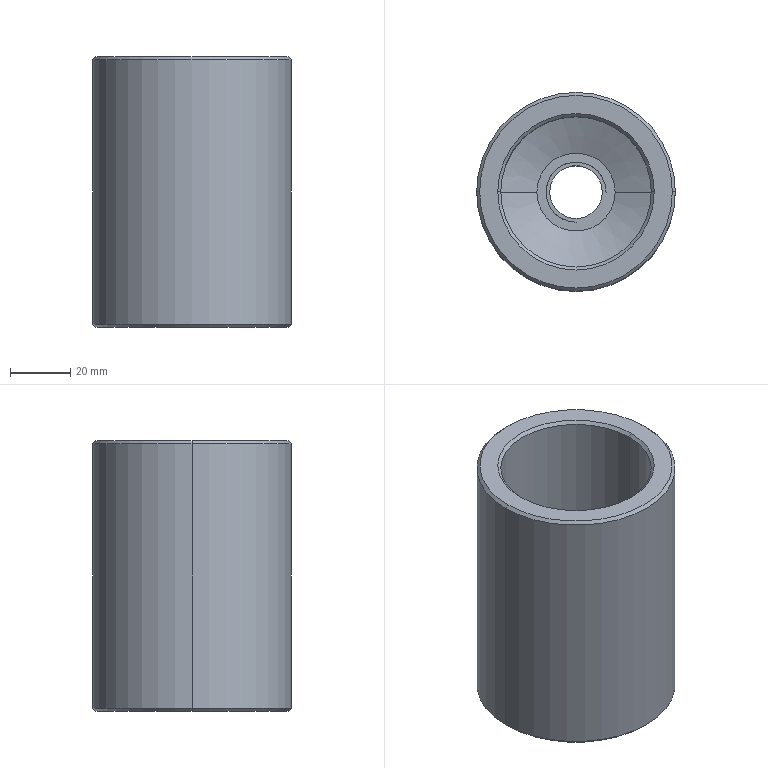Part | Creo | 1 solid | 21 faces | box 66 x 66 x 90 mm | volume 165854 mm3 | cone 8 | cylinder 8 | plane 5 | commonest cylinder face diameters 17.5 x2 50 x2 66 x2 19.94 x1 20 x1
STEP:
#1=CARTESIAN_POINT('',(-203.,-292.005,-366.));
#2=VERTEX_POINT('',#1);
#3=CARTESIAN_POINT('',(-267.,-292.005,-366.));
#4=VERTEX_POINT('',#3);
#5=CARTESIAN_POINT('',(-235.,-292.005,-366.));
#6=DIRECTION('',(0.,0.,-1.));
#7=DIRECTION('',(1.,0.,0.));
#8=AXIS2_PLACEMENT_3D('',#5,#6,#7);
#9=CIRCLE('',#8,32.);
#10=EDGE_CURVE('',#2,#4,#9,.T.);
#11=ORIENTED_EDGE('',*,*,#10,.F.);
#12=CARTESIAN_POINT('',(-235.,-292.005,-366.));
#13=DIRECTION('',(0.,0.,-1.));
#14=DIRECTION('',(-1.,0.,0.));
#15=AXIS2_PLACEMENT_3D('',#12,#13,#14);
#16=CIRCLE('',#15,32.);
#17=EDGE_CURVE('',#4,#2,#16,.T.);
#18=ORIENTED_EDGE('',*,*,#17,.F.);
#19=EDGE_LOOP('',(#11,#18));
#20=FACE_OUTER_BOUND('',#19,.F.);
#21=CARTESIAN_POINT('',(-225.03,-292.005,-366.));
#22=VERTEX_POINT('',#21);
#23=CARTESIAN_POINT('',(-225.,-292.005,-366.));
#24=VERTEX_POINT('',#23);
#25=CARTESIAN_POINT('',(-225.03,-292.005,-366.));
#26=DIRECTION('',(1.,0.,0.));
#27=VECTOR('',#26,0.03);
#28=LINE('',#25,#27);
#29=EDGE_CURVE('',#22,#24,#28,.T.);
#30=ORIENTED_EDGE('',*,*,#29,.F.);
#31=CARTESIAN_POINT('',(-244.97,-292.005,-366.));
#32=VERTEX_POINT('',#31);
#33=CARTESIAN_POINT('',(-235.,-292.005,-366.));
#34=DIRECTION('',(0.,0.,-1.));
#35=DIRECTION('',(-1.,0.,0.));
#36=AXIS2_PLACEMENT_3D('',#33,#34,#35);
#37=CIRCLE('',#36,9.97);
#38=EDGE_CURVE('',#32,#22,#37,.T.);
#39=ORIENTED_EDGE('',*,*,#38,.F.);
#40=CARTESIAN_POINT('',(-235.,-301.975,-366.));
#41=VERTEX_POINT('',#40);
#42=CARTESIAN_POINT('',(-235.,-292.005,-366.));
#43=DIRECTION('',(0.,0.,-1.));
#44=DIRECTION('',(0.,-1.,0.));
#45=AXIS2_PLACEMENT_3D('',#42,#43,#44);
#46=CIRCLE('',#45,9.97);
#47=EDGE_CURVE('',#41,#32,#46,.T.);
#48=ORIENTED_EDGE('',*,*,#47,.F.);
#49=CARTESIAN_POINT('',(-235.,-302.005,-366.));
#50=VERTEX_POINT('',#49);
#51=CARTESIAN_POINT('',(-235.,-302.005,-366.));
#52=DIRECTION('',(0.,1.,0.));
#53=VECTOR('',#52,0.03);
#54=LINE('',#51,#53);
#55=EDGE_CURVE('',#50,#41,#54,.T.);
#56=ORIENTED_EDGE('',*,*,#55,.F.);
#57=CARTESIAN_POINT('',(-245.,-292.005,-366.));
#58=VERTEX_POINT('',#57);
#59=CARTESIAN_POINT('',(-235.,-292.005,-366.));
#60=DIRECTION('',(0.,0.,1.));
#61=DIRECTION('',(-1.,0.,0.));
#62=AXIS2_PLACEMENT_3D('',#59,#60,#61);
#63=CIRCLE('',#62,10.);
#64=EDGE_CURVE('',#58,#50,#63,.T.);
#65=ORIENTED_EDGE('',*,*,#64,.F.);
#66=CARTESIAN_POINT('',(-235.,-292.005,-366.));
#67=DIRECTION('',(0.,0.,1.));
#68=DIRECTION('',(1.,0.,0.));
#69=AXIS2_PLACEMENT_3D('',#66,#67,#68);
#70=CIRCLE('',#69,10.);
#71=EDGE_CURVE('',#24,#58,#70,.T.);
#72=ORIENTED_EDGE('',*,*,#71,.F.);
#73=EDGE_LOOP('',(#30,#39,#48,#56,#65,#72));
#74=FACE_BOUND('',#73,.F.);
#75=CARTESIAN_POINT('',(-226.25,-292.005,-366.));
#76=VERTEX_POINT('',#75);
#77=CARTESIAN_POINT('',(-243.75,-292.005,-366.));
#78=VERTEX_POINT('',#77);
#79=CARTESIAN_POINT('',(-235.,-292.005,-366.));
#80=DIRECTION('',(0.,0.,1.));
#81=DIRECTION('',(1.,0.,0.));
#82=AXIS2_PLACEMENT_3D('',#79,#80,#81);
#83=CIRCLE('',#82,8.75);
#84=EDGE_CURVE('',#76,#78,#83,.T.);
#85=ORIENTED_EDGE('',*,*,#84,.F.);
#86=CARTESIAN_POINT('',(-235.,-292.005,-366.));
#87=DIRECTION('',(0.,0.,1.));
#88=DIRECTION('',(-1.,0.,0.));
#89=AXIS2_PLACEMENT_3D('',#86,#87,#88);
#90=CIRCLE('',#89,8.75);
#91=EDGE_CURVE('',#78,#76,#90,.T.);
#92=ORIENTED_EDGE('',*,*,#91,.F.);
#93=EDGE_LOOP('',(#85,#92));
#94=FACE_BOUND('',#93,.F.);
#95=CARTESIAN_POINT('',(-45.,-44.005,-366.));
#96=DIRECTION('',(0.,0.,-1.));
#97=DIRECTION('',(1.,0.,0.));
#98=AXIS2_PLACEMENT_3D('',#95,#96,#97);
#99=PLANE('',#98);
#100=ADVANCED_FACE('',(#20,#74,#94),#99,.T.);
#101=ORIENTED_EDGE('',*,*,#10,.T.);
#102=CARTESIAN_POINT('',(-268.,-292.005,-365.));
#103=VERTEX_POINT('',#102);
#104=CARTESIAN_POINT('',(-267.,-292.005,-366.));
#105=DIRECTION('',(-0.7071,0.,0.7071));
#106=VECTOR('',#105,1.414);
#107=LINE('',#104,#106);
#108=EDGE_CURVE('',#4,#103,#107,.T.);
#109=ORIENTED_EDGE('',*,*,#108,.T.);
#110=CARTESIAN_POINT('',(-202.,-292.005,-365.));
#111=VERTEX_POINT('',#110);
#112=CARTESIAN_POINT('',(-235.,-292.005,-365.));
#113=DIRECTION('',(0.,0.,-1.));
#114=DIRECTION('',(1.,0.,0.));
#115=AXIS2_PLACEMENT_3D('',#112,#113,#114);
#116=CIRCLE('',#115,33.);
#117=EDGE_CURVE('',#111,#103,#116,.T.);
#118=ORIENTED_EDGE('',*,*,#117,.F.);
#119=CARTESIAN_POINT('',(-203.,-292.005,-366.));
#120=DIRECTION('',(0.7071,0.,0.7071));
#121=VECTOR('',#120,1.414);
#122=LINE('',#119,#121);
#123=EDGE_CURVE('',#2,#111,#122,.T.);
#124=ORIENTED_EDGE('',*,*,#123,.F.);
#125=EDGE_LOOP('',(#101,#109,#118,#124));
#126=FACE_OUTER_BOUND('',#125,.F.);
#127=CARTESIAN_POINT('',(-235.,-292.005,-365.5));
#128=DIRECTION('',(0.,0.,1.));
#129=DIRECTION('',(-1.,0.,0.));
#130=AXIS2_PLACEMENT_3D('',#127,#128,#129);
#131=CONICAL_SURFACE('',#130,32.5,45.);
#132=ADVANCED_FACE('',(#126),#131,.T.);
#133=ORIENTED_EDGE('',*,*,#17,.T.);
#134=ORIENTED_EDGE('',*,*,#123,.T.);
#135=CARTESIAN_POINT('',(-235.,-292.005,-365.));
#136=DIRECTION('',(0.,0.,-1.));
#137=DIRECTION('',(-1.,0.,0.));
#138=AXIS2_PLACEMENT_3D('',#135,#136,#137);
#139=CIRCLE('',#138,33.);
#140=EDGE_CURVE('',#103,#111,#139,.T.);
#141=ORIENTED_EDGE('',*,*,#140,.F.);
#142=ORIENTED_EDGE('',*,*,#108,.F.);
#143=EDGE_LOOP('',(#133,#134,#141,#142));
#144=FACE_OUTER_BOUND('',#143,.F.);
#145=CARTESIAN_POINT('',(-235.,-292.005,-365.5));
#146=DIRECTION('',(0.,0.,1.));
#147=DIRECTION('',(-1.,0.,0.));
#148=AXIS2_PLACEMENT_3D('',#145,#146,#147);
#149=CONICAL_SURFACE('',#148,32.5,45.);
#150=ADVANCED_FACE('',(#144),#149,.T.);
#151=ORIENTED_EDGE('',*,*,#140,.T.);
#152=CARTESIAN_POINT('',(-202.,-292.005,-277.));
#153=VERTEX_POINT('',#152);
#154=CARTESIAN_POINT('',(-202.,-292.005,-277.));
#155=DIRECTION('',(0.,0.,-1.));
#156=VECTOR('',#155,88.);
#157=LINE('',#154,#156);
#158=EDGE_CURVE('',#153,#111,#157,.T.);
#159=ORIENTED_EDGE('',*,*,#158,.F.);
#160=CARTESIAN_POINT('',(-268.,-292.005,-277.));
#161=VERTEX_POINT('',#160);
#162=CARTESIAN_POINT('',(-235.,-292.005,-277.));
#163=DIRECTION('',(0.,0.,1.));
#164=DIRECTION('',(1.,0.,0.));
#165=AXIS2_PLACEMENT_3D('',#162,#163,#164);
#166=CIRCLE('',#165,33.);
#167=EDGE_CURVE('',#153,#161,#166,.T.);
#168=ORIENTED_EDGE('',*,*,#167,.T.);
#169=CARTESIAN_POINT('',(-268.,-292.005,-277.));
#170=DIRECTION('',(0.,0.,-1.));
#171=VECTOR('',#170,88.);
#172=LINE('',#169,#171);
#173=EDGE_CURVE('',#161,#103,#172,.T.);
#174=ORIENTED_EDGE('',*,*,#173,.T.);
#175=EDGE_LOOP('',(#151,#159,#168,#174));
#176=FACE_OUTER_BOUND('',#175,.F.);
#177=CARTESIAN_POINT('',(-235.,-292.005,-396.));
#178=DIRECTION('',(0.,0.,-1.));
#179=DIRECTION('',(1.,0.,0.));
#180=AXIS2_PLACEMENT_3D('',#177,#178,#179);
#181=CYLINDRICAL_SURFACE('',#180,33.);
#182=ADVANCED_FACE('',(#176),#181,.T.);
#183=ORIENTED_EDGE('',*,*,#117,.T.);
#184=ORIENTED_EDGE('',*,*,#173,.F.);
#185=CARTESIAN_POINT('',(-235.,-292.005,-277.));
#186=DIRECTION('',(0.,0.,1.));
#187=DIRECTION('',(-1.,0.,0.));
#188=AXIS2_PLACEMENT_3D('',#185,#186,#187);
#189=CIRCLE('',#188,33.);
#190=EDGE_CURVE('',#161,#153,#189,.T.);
#191=ORIENTED_EDGE('',*,*,#190,.T.);
#192=ORIENTED_EDGE('',*,*,#158,.T.);
#193=EDGE_LOOP('',(#183,#184,#191,#192));
#194=FACE_OUTER_BOUND('',#193,.F.);
#195=CARTESIAN_POINT('',(-235.,-292.005,-396.));
#196=DIRECTION('',(0.,0.,-1.));
#197=DIRECTION('',(1.,0.,0.));
#198=AXIS2_PLACEMENT_3D('',#195,#196,#197);
#199=CYLINDRICAL_SURFACE('',#198,33.);
#200=ADVANCED_FACE('',(#194),#199,.T.);
#201=CARTESIAN_POINT('',(-267.,-292.005,-276.));
#202=VERTEX_POINT('',#201);
#203=CARTESIAN_POINT('',(-203.,-292.005,-276.));
#204=VERTEX_POINT('',#203);
#205=CARTESIAN_POINT('',(-235.,-292.005,-276.));
#206=DIRECTION('',(0.,0.,1.));
#207=DIRECTION('',(-1.,0.,0.));
#208=AXIS2_PLACEMENT_3D('',#205,#206,#207);
#209=CIRCLE('',#208,32.);
#210=EDGE_CURVE('',#202,#204,#209,.T.);
#211=ORIENTED_EDGE('',*,*,#210,.T.);
#212=CARTESIAN_POINT('',(-203.,-292.005,-276.));
#213=DIRECTION('',(0.7071,0.,-0.7071));
#214=VECTOR('',#213,1.414);
#215=LINE('',#212,#214);
#216=EDGE_CURVE('',#204,#153,#215,.T.);
#217=ORIENTED_EDGE('',*,*,#216,.T.);
#218=ORIENTED_EDGE('',*,*,#190,.F.);
#219=CARTESIAN_POINT('',(-267.,-292.005,-276.));
#220=DIRECTION('',(-0.7071,0.,-0.7071));
#221=VECTOR('',#220,1.414);
#222=LINE('',#219,#221);
#223=EDGE_CURVE('',#202,#161,#222,.T.);
#224=ORIENTED_EDGE('',*,*,#223,.F.);
#225=EDGE_LOOP('',(#211,#217,#218,#224));
#226=FACE_OUTER_BOUND('',#225,.F.);
#227=CARTESIAN_POINT('',(-235.,-292.005,-276.5));
#228=DIRECTION('',(0.,0.,-1.));
#229=DIRECTION('',(-1.,0.,0.));
#230=AXIS2_PLACEMENT_3D('',#227,#228,#229);
#231=CONICAL_SURFACE('',#230,32.5,45.);
#232=ADVANCED_FACE('',(#226),#231,.T.);
#233=ORIENTED_EDGE('',*,*,#210,.F.);
#234=CARTESIAN_POINT('',(-235.,-292.005,-276.));
#235=DIRECTION('',(0.,0.,1.));
#236=DIRECTION('',(1.,0.,0.));
#237=AXIS2_PLACEMENT_3D('',#234,#235,#236);
#238=CIRCLE('',#237,32.);
#239=EDGE_CURVE('',#204,#202,#238,.T.);
#240=ORIENTED_EDGE('',*,*,#239,.F.);
#241=EDGE_LOOP('',(#233,#240));
#242=FACE_OUTER_BOUND('',#241,.F.);
#243=CARTESIAN_POINT('',(-209.,-292.005,-276.));
#244=VERTEX_POINT('',#243);
#245=CARTESIAN_POINT('',(-261.,-292.005,-276.));
#246=VERTEX_POINT('',#245);
#247=CARTESIAN_POINT('',(-235.,-292.005,-276.));
#248=DIRECTION('',(0.,0.,-1.));
#249=DIRECTION('',(1.,0.,0.));
#250=AXIS2_PLACEMENT_3D('',#247,#248,#249);
#251=CIRCLE('',#250,26.);
#252=EDGE_CURVE('',#244,#246,#251,.T.);
#253=ORIENTED_EDGE('',*,*,#252,.F.);
#254=CARTESIAN_POINT('',(-235.,-292.005,-276.));
#255=DIRECTION('',(0.,0.,-1.));
#256=DIRECTION('',(-1.,0.,0.));
#257=AXIS2_PLACEMENT_3D('',#254,#255,#256);
#258=CIRCLE('',#257,26.);
#259=EDGE_CURVE('',#246,#244,#258,.T.);
#260=ORIENTED_EDGE('',*,*,#259,.F.);
#261=EDGE_LOOP('',(#253,#260));
#262=FACE_BOUND('',#261,.F.);
#263=CARTESIAN_POINT('',(-45.,-44.005,-276.));
#264=DIRECTION('',(0.,0.,-1.));
#265=DIRECTION('',(1.,0.,0.));
#266=AXIS2_PLACEMENT_3D('',#263,#264,#265);
#267=PLANE('',#266);
#268=ADVANCED_FACE('',(#242,#262),#267,.F.);
#269=ORIENTED_EDGE('',*,*,#252,.T.);
#270=CARTESIAN_POINT('',(-260.,-292.005,-277.));
#271=VERTEX_POINT('',#270);
#272=CARTESIAN_POINT('',(-260.,-292.005,-277.));
#273=DIRECTION('',(-0.7071,0.,0.7071));
#274=VECTOR('',#273,1.414);
#275=LINE('',#272,#274);
#276=EDGE_CURVE('',#271,#246,#275,.T.);
#277=ORIENTED_EDGE('',*,*,#276,.F.);
#278=CARTESIAN_POINT('',(-210.,-292.005,-277.));
#279=VERTEX_POINT('',#278);
#280=CARTESIAN_POINT('',(-235.,-292.005,-277.));
#281=DIRECTION('',(0.,0.,-1.));
#282=DIRECTION('',(1.,0.,0.));
#283=AXIS2_PLACEMENT_3D('',#280,#281,#282);
#284=CIRCLE('',#283,25.);
#285=EDGE_CURVE('',#279,#271,#284,.T.);
#286=ORIENTED_EDGE('',*,*,#285,.F.);
#287=CARTESIAN_POINT('',(-210.,-292.005,-277.));
#288=DIRECTION('',(0.7071,0.,0.7071));
#289=VECTOR('',#288,1.414);
#290=LINE('',#287,#289);
#291=EDGE_CURVE('',#279,#244,#290,.T.);
#292=ORIENTED_EDGE('',*,*,#291,.T.);
#293=EDGE_LOOP('',(#269,#277,#286,#292));
#294=FACE_OUTER_BOUND('',#293,.F.);
#295=CARTESIAN_POINT('',(-235.,-292.005,-276.5));
#296=DIRECTION('',(0.,0.,1.));
#297=DIRECTION('',(-1.,0.,0.));
#298=AXIS2_PLACEMENT_3D('',#295,#296,#297);
#299=CONICAL_SURFACE('',#298,25.5,45.);
#300=ADVANCED_FACE('',(#294),#299,.F.);
#301=ORIENTED_EDGE('',*,*,#259,.T.);
#302=ORIENTED_EDGE('',*,*,#291,.F.);
#303=CARTESIAN_POINT('',(-235.,-292.005,-277.));
#304=DIRECTION('',(0.,0.,-1.));
#305=DIRECTION('',(-1.,0.,0.));
#306=AXIS2_PLACEMENT_3D('',#303,#304,#305);
#307=CIRCLE('',#306,25.);
#308=EDGE_CURVE('',#271,#279,#307,.T.);
#309=ORIENTED_EDGE('',*,*,#308,.F.);
#310=ORIENTED_EDGE('',*,*,#276,.T.);
#311=EDGE_LOOP('',(#301,#302,#309,#310));
#312=FACE_OUTER_BOUND('',#311,.F.);
#313=CARTESIAN_POINT('',(-235.,-292.005,-276.5));
#314=DIRECTION('',(0.,0.,1.));
#315=DIRECTION('',(-1.,0.,0.));
#316=AXIS2_PLACEMENT_3D('',#313,#314,#315);
#317=CONICAL_SURFACE('',#316,25.5,45.);
#318=ADVANCED_FACE('',(#312),#317,.F.);
#319=CARTESIAN_POINT('',(-210.,-292.005,-343.));
#320=VERTEX_POINT('',#319);
#321=CARTESIAN_POINT('',(-260.,-292.005,-343.));
#322=VERTEX_POINT('',#321);
#323=CARTESIAN_POINT('',(-235.,-292.005,-343.));
#324=DIRECTION('',(0.,0.,1.));
#325=DIRECTION('',(1.,0.,0.));
#326=AXIS2_PLACEMENT_3D('',#323,#324,#325);
#327=CIRCLE('',#326,25.);
#328=EDGE_CURVE('',#320,#322,#327,.T.);
#329=ORIENTED_EDGE('',*,*,#328,.T.);
#330=CARTESIAN_POINT('',(-260.,-292.005,-277.));
#331=DIRECTION('',(0.,0.,-1.));
#332=VECTOR('',#331,66.);
#333=LINE('',#330,#332);
#334=EDGE_CURVE('',#271,#322,#333,.T.);
#335=ORIENTED_EDGE('',*,*,#334,.F.);
#336=ORIENTED_EDGE('',*,*,#308,.T.);
#337=CARTESIAN_POINT('',(-210.,-292.005,-277.));
#338=DIRECTION('',(0.,0.,-1.));
#339=VECTOR('',#338,66.);
#340=LINE('',#337,#339);
#341=EDGE_CURVE('',#279,#320,#340,.T.);
#342=ORIENTED_EDGE('',*,*,#341,.T.);
#343=EDGE_LOOP('',(#329,#335,#336,#342));
#344=FACE_OUTER_BOUND('',#343,.F.);
#345=CARTESIAN_POINT('',(-235.,-292.005,-396.));
#346=DIRECTION('',(0.,0.,-1.));
#347=DIRECTION('',(1.,0.,0.));
#348=AXIS2_PLACEMENT_3D('',#345,#346,#347);
#349=CYLINDRICAL_SURFACE('',#348,25.);
#350=ADVANCED_FACE('',(#344),#349,.F.);
#351=ORIENTED_EDGE('',*,*,#328,.F.);
#352=CARTESIAN_POINT('',(-222.,-292.005,-348.));
#353=VERTEX_POINT('',#352);
#354=CARTESIAN_POINT('',(-222.,-292.005,-348.));
#355=DIRECTION('',(0.9231,0.,0.3846));
#356=VECTOR('',#355,13.);
#357=LINE('',#354,#356);
#358=EDGE_CURVE('',#353,#320,#357,.T.);
#359=ORIENTED_EDGE('',*,*,#358,.F.);
#360=CARTESIAN_POINT('',(-248.,-292.005,-348.));
#361=VERTEX_POINT('',#360);
#362=CARTESIAN_POINT('',(-235.,-292.005,-348.));
#363=DIRECTION('',(0.,0.,1.));
#364=DIRECTION('',(1.,0.,0.));
#365=AXIS2_PLACEMENT_3D('',#362,#363,#364);
#366=CIRCLE('',#365,13.);
#367=EDGE_CURVE('',#353,#361,#366,.T.);
#368=ORIENTED_EDGE('',*,*,#367,.T.);
#369=CARTESIAN_POINT('',(-248.,-292.005,-348.));
#370=DIRECTION('',(-0.9231,0.,0.3846));
#371=VECTOR('',#370,13.);
#372=LINE('',#369,#371);
#373=EDGE_CURVE('',#361,#322,#372,.T.);
#374=ORIENTED_EDGE('',*,*,#373,.T.);
#375=EDGE_LOOP('',(#351,#359,#368,#374));
#376=FACE_OUTER_BOUND('',#375,.F.);
#377=CARTESIAN_POINT('',(-235.,-292.005,-345.5));
#378=DIRECTION('',(0.,0.,1.));
#379=DIRECTION('',(-1.,0.,0.));
#380=AXIS2_PLACEMENT_3D('',#377,#378,#379);
#381=CONICAL_SURFACE('',#380,19.,67.38);
#382=ADVANCED_FACE('',(#376),#381,.F.);
#383=CARTESIAN_POINT('',(-235.,-292.005,-343.));
#384=DIRECTION('',(0.,0.,1.));
#385=DIRECTION('',(-1.,0.,0.));
#386=AXIS2_PLACEMENT_3D('',#383,#384,#385);
#387=CIRCLE('',#386,25.);
#388=EDGE_CURVE('',#322,#320,#387,.T.);
#389=ORIENTED_EDGE('',*,*,#388,.F.);
#390=ORIENTED_EDGE('',*,*,#373,.F.);
#391=CARTESIAN_POINT('',(-235.,-292.005,-348.));
#392=DIRECTION('',(0.,0.,1.));
#393=DIRECTION('',(-1.,0.,0.));
#394=AXIS2_PLACEMENT_3D('',#391,#392,#393);
#395=CIRCLE('',#394,13.);
#396=EDGE_CURVE('',#361,#353,#395,.T.);
#397=ORIENTED_EDGE('',*,*,#396,.T.);
#398=ORIENTED_EDGE('',*,*,#358,.T.);
#399=EDGE_LOOP('',(#389,#390,#397,#398));
#400=FACE_OUTER_BOUND('',#399,.F.);
#401=CARTESIAN_POINT('',(-235.,-292.005,-345.5));
#402=DIRECTION('',(0.,0.,1.));
#403=DIRECTION('',(-1.,0.,0.));
#404=AXIS2_PLACEMENT_3D('',#401,#402,#403);
#405=CONICAL_SURFACE('',#404,19.,67.38);
#406=ADVANCED_FACE('',(#400),#405,.F.);
#407=ORIENTED_EDGE('',*,*,#388,.T.);
#408=ORIENTED_EDGE('',*,*,#341,.F.);
#409=ORIENTED_EDGE('',*,*,#285,.T.);
#410=ORIENTED_EDGE('',*,*,#334,.T.);
#411=EDGE_LOOP('',(#407,#408,#409,#410));
#412=FACE_OUTER_BOUND('',#411,.F.);
#413=CARTESIAN_POINT('',(-235.,-292.005,-396.));
#414=DIRECTION('',(0.,0.,-1.));
#415=DIRECTION('',(1.,0.,0.));
#416=AXIS2_PLACEMENT_3D('',#413,#414,#415);
#417=CYLINDRICAL_SURFACE('',#416,25.);
#418=ADVANCED_FACE('',(#412),#417,.F.);
#419=ORIENTED_EDGE('',*,*,#396,.F.);
#420=ORIENTED_EDGE('',*,*,#367,.F.);
#421=EDGE_LOOP('',(#419,#420));
#422=FACE_OUTER_BOUND('',#421,.F.);
#423=CARTESIAN_POINT('',(-243.75,-292.005,-348.));
#424=VERTEX_POINT('',#423);
#425=CARTESIAN_POINT('',(-226.25,-292.005,-348.));
#426=VERTEX_POINT('',#425);
#427=CARTESIAN_POINT('',(-235.,-292.005,-348.));
#428=DIRECTION('',(0.,0.,-1.));
#429=DIRECTION('',(-1.,0.,0.));
#430=AXIS2_PLACEMENT_3D('',#427,#428,#429);
#431=CIRCLE('',#430,8.75);
#432=EDGE_CURVE('',#424,#426,#431,.T.);
#433=ORIENTED_EDGE('',*,*,#432,.F.);
#434=CARTESIAN_POINT('',(-235.,-292.005,-348.));
#435=DIRECTION('',(0.,0.,-1.));
#436=DIRECTION('',(1.,0.,0.));
#437=AXIS2_PLACEMENT_3D('',#434,#435,#436);
#438=CIRCLE('',#437,8.75);
#439=EDGE_CURVE('',#426,#424,#438,.T.);
#440=ORIENTED_EDGE('',*,*,#439,.F.);
#441=EDGE_LOOP('',(#433,#440));
#442=FACE_BOUND('',#441,.F.);
#443=CARTESIAN_POINT('',(-235.,-301.975,-348.));
#444=VERTEX_POINT('',#443);
#445=CARTESIAN_POINT('',(-235.,-302.005,-348.));
#446=VERTEX_POINT('',#445);
#447=CARTESIAN_POINT('',(-235.,-301.975,-348.));
#448=DIRECTION('',(0.,-1.,0.));
#449=VECTOR('',#448,0.03);
#450=LINE('',#447,#449);
#451=EDGE_CURVE('',#444,#446,#450,.T.);
#452=ORIENTED_EDGE('',*,*,#451,.F.);
#453=CARTESIAN_POINT('',(-225.03,-292.005,-348.));
#454=VERTEX_POINT('',#453);
#455=CARTESIAN_POINT('',(-235.,-292.005,-348.));
#456=DIRECTION('',(0.,0.,1.));
#457=DIRECTION('',(1.,0.,0.));
#458=AXIS2_PLACEMENT_3D('',#455,#456,#457);
#459=CIRCLE('',#458,9.97);
#460=EDGE_CURVE('',#454,#444,#459,.T.);
#461=ORIENTED_EDGE('',*,*,#460,.F.);
#462=CARTESIAN_POINT('',(-225.,-292.005,-348.));
#463=VERTEX_POINT('',#462);
#464=CARTESIAN_POINT('',(-225.,-292.005,-348.));
#465=DIRECTION('',(-1.,0.,0.));
#466=VECTOR('',#465,0.03);
#467=LINE('',#464,#466);
#468=EDGE_CURVE('',#463,#454,#467,.T.);
#469=ORIENTED_EDGE('',*,*,#468,.F.);
#470=CARTESIAN_POINT('',(-235.,-292.005,-348.));
#471=DIRECTION('',(0.,0.,-1.));
#472=DIRECTION('',(0.,-1.,0.));
#473=AXIS2_PLACEMENT_3D('',#470,#471,#472);
#474=CIRCLE('',#473,10.);
#475=EDGE_CURVE('',#446,#463,#474,.T.);
#476=ORIENTED_EDGE('',*,*,#475,.F.);
#477=EDGE_LOOP('',(#452,#461,#469,#476));
#478=FACE_BOUND('',#477,.F.);
#479=CARTESIAN_POINT('',(-45.,-44.005,-348.));
#480=DIRECTION('',(0.,0.,-1.));
#481=DIRECTION('',(0.,1.,0.));
#482=AXIS2_PLACEMENT_3D('',#479,#480,#481);
#483=PLANE('',#482);
#484=ADVANCED_FACE('',(#422,#442,#478),#483,.F.);
#485=ORIENTED_EDGE('',*,*,#84,.T.);
#486=CARTESIAN_POINT('',(-243.75,-292.005,-366.));
#487=DIRECTION('',(0.,0.,1.));
#488=VECTOR('',#487,18.);
#489=LINE('',#486,#488);
#490=EDGE_CURVE('',#78,#424,#489,.T.);
#491=ORIENTED_EDGE('',*,*,#490,.T.);
#492=ORIENTED_EDGE('',*,*,#432,.T.);
#493=CARTESIAN_POINT('',(-226.25,-292.005,-366.));
#494=DIRECTION('',(0.,0.,1.));
#495=VECTOR('',#494,18.);
#496=LINE('',#493,#495);
#497=EDGE_CURVE('',#76,#426,#496,.T.);
#498=ORIENTED_EDGE('',*,*,#497,.F.);
#499=EDGE_LOOP('',(#485,#491,#492,#498));
#500=FACE_OUTER_BOUND('',#499,.F.);
#501=CARTESIAN_POINT('',(-235.,-292.005,-366.));
#502=DIRECTION('',(0.,0.,1.));
#503=DIRECTION('',(1.,0.,0.));
#504=AXIS2_PLACEMENT_3D('',#501,#502,#503);
#505=CYLINDRICAL_SURFACE('',#504,8.75);
#506=ADVANCED_FACE('',(#500),#505,.F.);
#507=ORIENTED_EDGE('',*,*,#91,.T.);
#508=ORIENTED_EDGE('',*,*,#497,.T.);
#509=ORIENTED_EDGE('',*,*,#439,.T.);
#510=ORIENTED_EDGE('',*,*,#490,.F.);
#511=EDGE_LOOP('',(#507,#508,#509,#510));
#512=FACE_OUTER_BOUND('',#511,.F.);
#513=CARTESIAN_POINT('',(-235.,-292.005,-366.));
#514=DIRECTION('',(0.,0.,1.));
#515=DIRECTION('',(1.,0.,0.));
#516=AXIS2_PLACEMENT_3D('',#513,#514,#515);
#517=CYLINDRICAL_SURFACE('',#516,8.75);
#518=ADVANCED_FACE('',(#512),#517,.F.);
#519=ORIENTED_EDGE('',*,*,#451,.T.);
#520=CARTESIAN_POINT('',(-235.,-302.005,-348.));
#521=DIRECTION('',(0.,0.,-1.));
#522=VECTOR('',#521,18.);
#523=LINE('',#520,#522);
#524=EDGE_CURVE('',#446,#50,#523,.T.);
#525=ORIENTED_EDGE('',*,*,#524,.T.);
#526=ORIENTED_EDGE('',*,*,#55,.T.);
#527=CARTESIAN_POINT('',(-235.,-301.975,-366.));
#528=DIRECTION('',(0.,0.,1.));
#529=VECTOR('',#528,18.);
#530=LINE('',#527,#529);
#531=EDGE_CURVE('',#41,#444,#530,.T.);
#532=ORIENTED_EDGE('',*,*,#531,.T.);
#533=EDGE_LOOP('',(#519,#525,#526,#532));
#534=FACE_OUTER_BOUND('',#533,.F.);
#535=CARTESIAN_POINT('',(-235.,-297.005,-321.));
#536=DIRECTION('',(-1.,0.,0.));
#537=DIRECTION('',(0.,0.,-1.));
#538=AXIS2_PLACEMENT_3D('',#535,#536,#537);
#539=PLANE('',#538);
#540=ADVANCED_FACE('',(#534),#539,.T.);
#541=ORIENTED_EDGE('',*,*,#524,.F.);
#542=ORIENTED_EDGE('',*,*,#475,.T.);
#543=CARTESIAN_POINT('',(-225.,-292.005,-366.));
#544=DIRECTION('',(0.,0.,1.));
#545=VECTOR('',#544,18.);
#546=LINE('',#543,#545);
#547=EDGE_CURVE('',#24,#463,#546,.T.);
#548=ORIENTED_EDGE('',*,*,#547,.F.);
#549=ORIENTED_EDGE('',*,*,#71,.T.);
#550=ORIENTED_EDGE('',*,*,#64,.T.);
#551=EDGE_LOOP('',(#541,#542,#548,#549,#550));
#552=FACE_OUTER_BOUND('',#551,.F.);
#553=CARTESIAN_POINT('',(-235.,-292.005,-366.));
#554=DIRECTION('',(0.,0.,1.));
#555=DIRECTION('',(1.,0.,0.));
#556=AXIS2_PLACEMENT_3D('',#553,#554,#555);
#557=CYLINDRICAL_SURFACE('',#556,10.);
#558=ADVANCED_FACE('',(#552),#557,.F.);
#559=ORIENTED_EDGE('',*,*,#468,.T.);
#560=CARTESIAN_POINT('',(-225.03,-292.005,-348.));
#561=DIRECTION('',(0.,0.,-1.));
#562=VECTOR('',#561,18.);
#563=LINE('',#560,#562);
#564=EDGE_CURVE('',#454,#22,#563,.T.);
#565=ORIENTED_EDGE('',*,*,#564,.T.);
#566=ORIENTED_EDGE('',*,*,#29,.T.);
#567=ORIENTED_EDGE('',*,*,#547,.T.);
#568=EDGE_LOOP('',(#559,#565,#566,#567));
#569=FACE_OUTER_BOUND('',#568,.F.);
#570=CARTESIAN_POINT('',(-230.,-292.005,-321.));
#571=DIRECTION('',(0.,1.,0.));
#572=DIRECTION('',(0.,0.,1.));
#573=AXIS2_PLACEMENT_3D('',#570,#571,#572);
#574=PLANE('',#573);
#575=ADVANCED_FACE('',(#569),#574,.T.);
#576=ORIENTED_EDGE('',*,*,#460,.T.);
#577=ORIENTED_EDGE('',*,*,#531,.F.);
#578=ORIENTED_EDGE('',*,*,#47,.T.);
#579=ORIENTED_EDGE('',*,*,#38,.T.);
#580=ORIENTED_EDGE('',*,*,#564,.F.);
#581=EDGE_LOOP('',(#576,#577,#578,#579,#580));
#582=FACE_OUTER_BOUND('',#581,.F.);
#583=CARTESIAN_POINT('',(-235.,-292.005,-366.));
#584=DIRECTION('',(0.,0.,1.));
#585=DIRECTION('',(1.,0.,0.));
#586=AXIS2_PLACEMENT_3D('',#583,#584,#585);
#587=CYLINDRICAL_SURFACE('',#586,9.97);
#588=ADVANCED_FACE('',(#582),#587,.T.);
#589=ORIENTED_EDGE('',*,*,#239,.T.);
#590=ORIENTED_EDGE('',*,*,#223,.T.);
#591=ORIENTED_EDGE('',*,*,#167,.F.);
#592=ORIENTED_EDGE('',*,*,#216,.F.);
#593=EDGE_LOOP('',(#589,#590,#591,#592));
#594=FACE_OUTER_BOUND('',#593,.F.);
#595=CARTESIAN_POINT('',(-235.,-292.005,-276.5));
#596=DIRECTION('',(0.,0.,-1.));
#597=DIRECTION('',(-1.,0.,0.));
#598=AXIS2_PLACEMENT_3D('',#595,#596,#597);
#599=CONICAL_SURFACE('',#598,32.5,45.);
#600=ADVANCED_FACE('',(#594),#599,.T.);
#601=CLOSED_SHELL('',(#100,#132,#150,#182,#200,#232,#268,#300,#318,#350,#382,#406,#418,#484,#506,#518,#540,#558,#575,#588,#600));
#602=MANIFOLD_SOLID_BREP('',#601);
#603=(LENGTH_UNIT()NAMED_UNIT(*)SI_UNIT(.MILLI.,.METRE.));
#604=UNCERTAINTY_MEASURE_WITH_UNIT(LENGTH_MEASURE(0.01297),#603,'','');
#605=(NAMED_UNIT(*)PLANE_ANGLE_UNIT()SI_UNIT($,.RADIAN.));
#606=PLANE_ANGLE_MEASURE_WITH_UNIT(PLANE_ANGLE_MEASURE(0.01745),#605);
#607=(CONVERSION_BASED_UNIT('DEGREE',#606)NAMED_UNIT(*)PLANE_ANGLE_UNIT());
#608=(NAMED_UNIT(*)SI_UNIT($,.STERADIAN.)SOLID_ANGLE_UNIT());
#609=(GEOMETRIC_REPRESENTATION_CONTEXT(3)GLOBAL_UNCERTAINTY_ASSIGNED_CONTEXT((#604))GLOBAL_UNIT_ASSIGNED_CONTEXT((#603,#607,#608))REPRESENTATION_CONTEXT('',''));
#610=ADVANCED_BREP_SHAPE_REPRESENTATION('',(#602),#609);